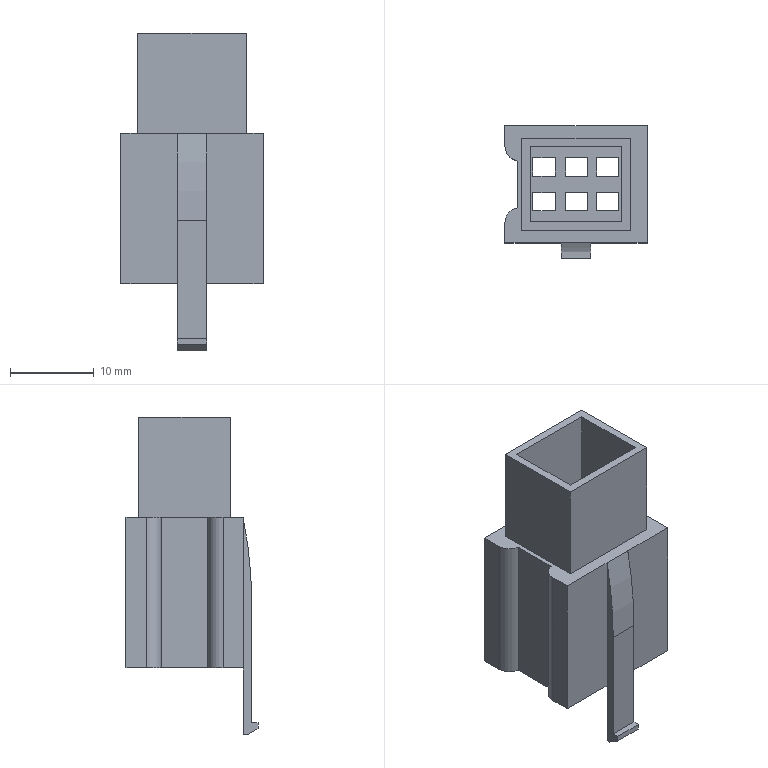Part | SolidWorks | features BaseBody 1 | 1 solid | 63 faces | box 17 x 15.786 x 38 mm | volume 1826 mm3 | plane 58 | cylinder 5 | commonest cylinder face diameters 1.689 x2 3.689 x2 104.893 x1